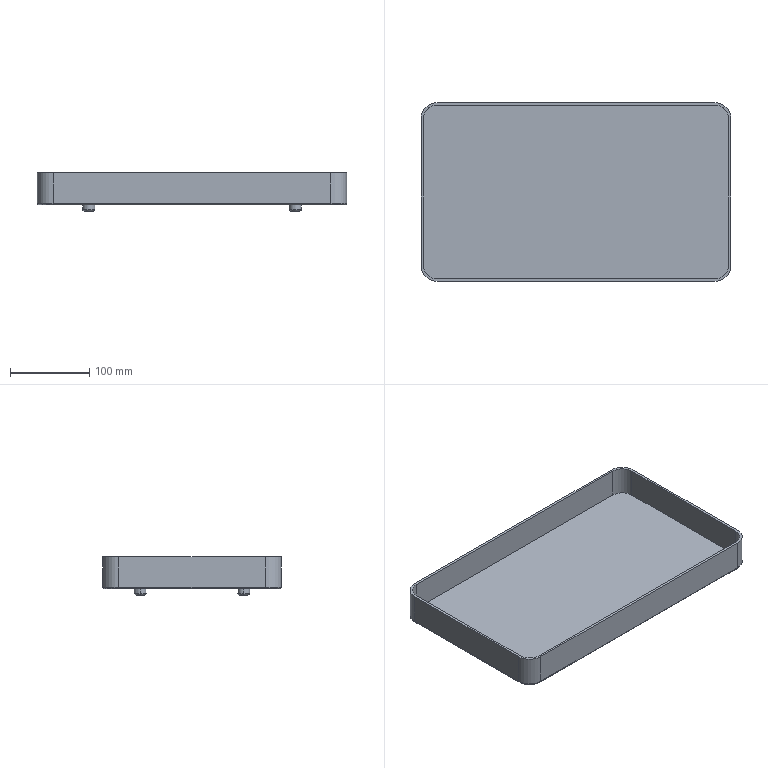Part | SolidWorks | features Fillet 3, Extrusion 1, ICE 1, LPattern 1, Shell 1 | 1 solid | 47 faces | box 390 x 225 x 48 mm | volume 398371 mm3 | cylinder 20 | plane 15 | torus 12 | commonest cylinder face diameters 15 x8 4 x4 34 x4 40 x4
STEP:
#1=CARTESIAN_POINT('',(-122.5,65.,-6.));
#2=VERTEX_POINT('',#1);
#3=CARTESIAN_POINT('',(-137.5,65.,-6.));
#4=VERTEX_POINT('',#3);
#5=CARTESIAN_POINT('',(-130.,65.,-6.));
#6=DIRECTION('',(0.,0.,1.));
#7=DIRECTION('',(-1.,0.,0.));
#8=AXIS2_PLACEMENT_3D('',#5,#6,#7);
#9=CIRCLE('',#8,7.5);
#10=EDGE_CURVE('',#2,#4,#9,.T.);
#11=ORIENTED_EDGE('',*,*,#10,.F.);
#12=CARTESIAN_POINT('',(-124.5,65.,-8.));
#13=VERTEX_POINT('',#12);
#14=CARTESIAN_POINT('',(-124.5,65.,-6.));
#15=DIRECTION('',(0.,1.,0.));
#16=DIRECTION('',(-1.,0.,0.));
#17=AXIS2_PLACEMENT_3D('',#14,#15,#16);
#18=CIRCLE('',#17,2.);
#19=EDGE_CURVE('',#2,#13,#18,.T.);
#20=ORIENTED_EDGE('',*,*,#19,.T.);
#21=CARTESIAN_POINT('',(-135.5,65.,-8.));
#22=VERTEX_POINT('',#21);
#23=CARTESIAN_POINT('',(-130.,65.,-8.));
#24=DIRECTION('',(0.,0.,-1.));
#25=DIRECTION('',(-1.,0.,0.));
#26=AXIS2_PLACEMENT_3D('',#23,#24,#25);
#27=CIRCLE('',#26,5.5);
#28=EDGE_CURVE('',#22,#13,#27,.T.);
#29=ORIENTED_EDGE('',*,*,#28,.F.);
#30=CARTESIAN_POINT('',(-135.5,65.,-6.));
#31=DIRECTION('',(0.,-1.,0.));
#32=DIRECTION('',(0.,0.,-1.));
#33=AXIS2_PLACEMENT_3D('',#30,#31,#32);
#34=CIRCLE('',#33,2.);
#35=EDGE_CURVE('',#4,#22,#34,.T.);
#36=ORIENTED_EDGE('',*,*,#35,.F.);
#37=EDGE_LOOP('',(#11,#20,#29,#36));
#38=FACE_OUTER_BOUND('',#37,.T.);
#39=CARTESIAN_POINT('',(-130.,65.,-6.));
#40=DIRECTION('',(0.,0.,-1.));
#41=DIRECTION('',(-1.,0.,0.));
#42=AXIS2_PLACEMENT_3D('',#39,#40,#41);
#43=TOROIDAL_SURFACE('',#42,5.5,2.);
#44=ADVANCED_FACE('',(#38),#43,.T.);
#45=ORIENTED_EDGE('',*,*,#10,.T.);
#46=CARTESIAN_POINT('',(-137.5,65.,0.));
#47=VERTEX_POINT('',#46);
#48=CARTESIAN_POINT('',(-137.5,65.,-8.));
#49=DIRECTION('',(0.,0.,1.));
#50=VECTOR('',#49,1000.);
#51=LINE('',#48,#50);
#52=EDGE_CURVE('',#4,#47,#51,.T.);
#53=ORIENTED_EDGE('',*,*,#52,.T.);
#54=CARTESIAN_POINT('',(-122.5,65.,0.));
#55=VERTEX_POINT('',#54);
#56=CARTESIAN_POINT('',(-130.,65.,0.));
#57=DIRECTION('',(0.,0.,-1.));
#58=DIRECTION('',(-1.,0.,0.));
#59=AXIS2_PLACEMENT_3D('',#56,#57,#58);
#60=CIRCLE('',#59,7.5);
#61=EDGE_CURVE('',#47,#55,#60,.T.);
#62=ORIENTED_EDGE('',*,*,#61,.T.);
#63=CARTESIAN_POINT('',(-122.5,65.,-8.));
#64=DIRECTION('',(0.,0.,1.));
#65=VECTOR('',#64,1000.);
#66=LINE('',#63,#65);
#67=EDGE_CURVE('',#2,#55,#66,.T.);
#68=ORIENTED_EDGE('',*,*,#67,.F.);
#69=EDGE_LOOP('',(#45,#53,#62,#68));
#70=FACE_OUTER_BOUND('',#69,.T.);
#71=CARTESIAN_POINT('',(-130.,65.,-8.));
#72=DIRECTION('',(0.,0.,1.));
#73=DIRECTION('',(1.,0.,0.));
#74=AXIS2_PLACEMENT_3D('',#71,#72,#73);
#75=CYLINDRICAL_SURFACE('',#74,7.5);
#76=ADVANCED_FACE('',(#70),#75,.T.);
#77=CARTESIAN_POINT('',(137.5,65.,-6.));
#78=VERTEX_POINT('',#77);
#79=CARTESIAN_POINT('',(122.5,65.,-6.));
#80=VERTEX_POINT('',#79);
#81=CARTESIAN_POINT('',(130.,65.,-6.));
#82=DIRECTION('',(0.,0.,1.));
#83=DIRECTION('',(-1.,0.,0.));
#84=AXIS2_PLACEMENT_3D('',#81,#82,#83);
#85=CIRCLE('',#84,7.5);
#86=EDGE_CURVE('',#78,#80,#85,.T.);
#87=ORIENTED_EDGE('',*,*,#86,.F.);
#88=CARTESIAN_POINT('',(135.5,65.,-8.));
#89=VERTEX_POINT('',#88);
#90=CARTESIAN_POINT('',(135.5,65.,-6.));
#91=DIRECTION('',(0.,1.,0.));
#92=DIRECTION('',(-1.,0.,0.));
#93=AXIS2_PLACEMENT_3D('',#90,#91,#92);
#94=CIRCLE('',#93,2.);
#95=EDGE_CURVE('',#78,#89,#94,.T.);
#96=ORIENTED_EDGE('',*,*,#95,.T.);
#97=CARTESIAN_POINT('',(124.5,65.,-8.));
#98=VERTEX_POINT('',#97);
#99=CARTESIAN_POINT('',(130.,65.,-8.));
#100=DIRECTION('',(0.,0.,-1.));
#101=DIRECTION('',(-1.,0.,0.));
#102=AXIS2_PLACEMENT_3D('',#99,#100,#101);
#103=CIRCLE('',#102,5.5);
#104=EDGE_CURVE('',#98,#89,#103,.T.);
#105=ORIENTED_EDGE('',*,*,#104,.F.);
#106=CARTESIAN_POINT('',(124.5,65.,-6.));
#107=DIRECTION('',(0.,-1.,0.));
#108=DIRECTION('',(0.,0.,-1.));
#109=AXIS2_PLACEMENT_3D('',#106,#107,#108);
#110=CIRCLE('',#109,2.);
#111=EDGE_CURVE('',#80,#98,#110,.T.);
#112=ORIENTED_EDGE('',*,*,#111,.F.);
#113=EDGE_LOOP('',(#87,#96,#105,#112));
#114=FACE_OUTER_BOUND('',#113,.T.);
#115=CARTESIAN_POINT('',(130.,65.,-6.));
#116=DIRECTION('',(0.,0.,-1.));
#117=DIRECTION('',(-1.,0.,0.));
#118=AXIS2_PLACEMENT_3D('',#115,#116,#117);
#119=TOROIDAL_SURFACE('',#118,5.5,2.);
#120=ADVANCED_FACE('',(#114),#119,.T.);
#121=ORIENTED_EDGE('',*,*,#86,.T.);
#122=CARTESIAN_POINT('',(122.5,65.,0.));
#123=VERTEX_POINT('',#122);
#124=CARTESIAN_POINT('',(122.5,65.,-8.));
#125=DIRECTION('',(0.,0.,1.));
#126=VECTOR('',#125,1000.);
#127=LINE('',#124,#126);
#128=EDGE_CURVE('',#80,#123,#127,.T.);
#129=ORIENTED_EDGE('',*,*,#128,.T.);
#130=CARTESIAN_POINT('',(137.5,65.,0.));
#131=VERTEX_POINT('',#130);
#132=CARTESIAN_POINT('',(130.,65.,0.));
#133=DIRECTION('',(0.,0.,-1.));
#134=DIRECTION('',(-1.,0.,0.));
#135=AXIS2_PLACEMENT_3D('',#132,#133,#134);
#136=CIRCLE('',#135,7.5);
#137=EDGE_CURVE('',#123,#131,#136,.T.);
#138=ORIENTED_EDGE('',*,*,#137,.T.);
#139=CARTESIAN_POINT('',(137.5,65.,-8.));
#140=DIRECTION('',(0.,0.,1.));
#141=VECTOR('',#140,1000.);
#142=LINE('',#139,#141);
#143=EDGE_CURVE('',#78,#131,#142,.T.);
#144=ORIENTED_EDGE('',*,*,#143,.F.);
#145=EDGE_LOOP('',(#121,#129,#138,#144));
#146=FACE_OUTER_BOUND('',#145,.T.);
#147=CARTESIAN_POINT('',(130.,65.,-8.));
#148=DIRECTION('',(0.,0.,1.));
#149=DIRECTION('',(1.,0.,0.));
#150=AXIS2_PLACEMENT_3D('',#147,#148,#149);
#151=CYLINDRICAL_SURFACE('',#150,7.5);
#152=ADVANCED_FACE('',(#146),#151,.T.);
#153=CARTESIAN_POINT('',(137.5,-65.,-6.));
#154=VERTEX_POINT('',#153);
#155=CARTESIAN_POINT('',(122.5,-65.,-6.));
#156=VERTEX_POINT('',#155);
#157=CARTESIAN_POINT('',(130.,-65.,-6.));
#158=DIRECTION('',(0.,0.,1.));
#159=DIRECTION('',(-1.,0.,0.));
#160=AXIS2_PLACEMENT_3D('',#157,#158,#159);
#161=CIRCLE('',#160,7.5);
#162=EDGE_CURVE('',#154,#156,#161,.T.);
#163=ORIENTED_EDGE('',*,*,#162,.T.);
#164=CARTESIAN_POINT('',(122.5,-65.,0.));
#165=VERTEX_POINT('',#164);
#166=CARTESIAN_POINT('',(122.5,-65.,-8.));
#167=DIRECTION('',(0.,0.,1.));
#168=VECTOR('',#167,1000.);
#169=LINE('',#166,#168);
#170=EDGE_CURVE('',#156,#165,#169,.T.);
#171=ORIENTED_EDGE('',*,*,#170,.T.);
#172=CARTESIAN_POINT('',(137.5,-65.,0.));
#173=VERTEX_POINT('',#172);
#174=CARTESIAN_POINT('',(130.,-65.,0.));
#175=DIRECTION('',(0.,0.,-1.));
#176=DIRECTION('',(-1.,0.,0.));
#177=AXIS2_PLACEMENT_3D('',#174,#175,#176);
#178=CIRCLE('',#177,7.5);
#179=EDGE_CURVE('',#165,#173,#178,.T.);
#180=ORIENTED_EDGE('',*,*,#179,.T.);
#181=CARTESIAN_POINT('',(137.5,-65.,-8.));
#182=DIRECTION('',(0.,0.,1.));
#183=VECTOR('',#182,1000.);
#184=LINE('',#181,#183);
#185=EDGE_CURVE('',#154,#173,#184,.T.);
#186=ORIENTED_EDGE('',*,*,#185,.F.);
#187=EDGE_LOOP('',(#163,#171,#180,#186));
#188=FACE_OUTER_BOUND('',#187,.T.);
#189=CARTESIAN_POINT('',(130.,-65.,-8.));
#190=DIRECTION('',(0.,0.,1.));
#191=DIRECTION('',(1.,0.,0.));
#192=AXIS2_PLACEMENT_3D('',#189,#190,#191);
#193=CYLINDRICAL_SURFACE('',#192,7.5);
#194=ADVANCED_FACE('',(#188),#193,.T.);
#195=ORIENTED_EDGE('',*,*,#162,.F.);
#196=CARTESIAN_POINT('',(135.5,-65.,-8.));
#197=VERTEX_POINT('',#196);
#198=CARTESIAN_POINT('',(135.5,-65.,-6.));
#199=DIRECTION('',(0.,1.,0.));
#200=DIRECTION('',(-1.,0.,0.));
#201=AXIS2_PLACEMENT_3D('',#198,#199,#200);
#202=CIRCLE('',#201,2.);
#203=EDGE_CURVE('',#154,#197,#202,.T.);
#204=ORIENTED_EDGE('',*,*,#203,.T.);
#205=CARTESIAN_POINT('',(124.5,-65.,-8.));
#206=VERTEX_POINT('',#205);
#207=CARTESIAN_POINT('',(130.,-65.,-8.));
#208=DIRECTION('',(0.,0.,-1.));
#209=DIRECTION('',(-1.,0.,0.));
#210=AXIS2_PLACEMENT_3D('',#207,#208,#209);
#211=CIRCLE('',#210,5.5);
#212=EDGE_CURVE('',#206,#197,#211,.T.);
#213=ORIENTED_EDGE('',*,*,#212,.F.);
#214=CARTESIAN_POINT('',(124.5,-65.,-6.));
#215=DIRECTION('',(0.,-1.,0.));
#216=DIRECTION('',(0.,0.,-1.));
#217=AXIS2_PLACEMENT_3D('',#214,#215,#216);
#218=CIRCLE('',#217,2.);
#219=EDGE_CURVE('',#156,#206,#218,.T.);
#220=ORIENTED_EDGE('',*,*,#219,.F.);
#221=EDGE_LOOP('',(#195,#204,#213,#220));
#222=FACE_OUTER_BOUND('',#221,.T.);
#223=CARTESIAN_POINT('',(130.,-65.,-6.));
#224=DIRECTION('',(0.,0.,-1.));
#225=DIRECTION('',(-1.,0.,0.));
#226=AXIS2_PLACEMENT_3D('',#223,#224,#225);
#227=TOROIDAL_SURFACE('',#226,5.5,2.);
#228=ADVANCED_FACE('',(#222),#227,.T.);
#229=CARTESIAN_POINT('',(-122.5,-65.,-6.));
#230=VERTEX_POINT('',#229);
#231=CARTESIAN_POINT('',(-137.5,-65.,-6.));
#232=VERTEX_POINT('',#231);
#233=CARTESIAN_POINT('',(-130.,-65.,-6.));
#234=DIRECTION('',(0.,0.,1.));
#235=DIRECTION('',(-1.,0.,0.));
#236=AXIS2_PLACEMENT_3D('',#233,#234,#235);
#237=CIRCLE('',#236,7.5);
#238=EDGE_CURVE('',#230,#232,#237,.T.);
#239=ORIENTED_EDGE('',*,*,#238,.T.);
#240=CARTESIAN_POINT('',(-137.5,-65.,0.));
#241=VERTEX_POINT('',#240);
#242=CARTESIAN_POINT('',(-137.5,-65.,-8.));
#243=DIRECTION('',(0.,0.,1.));
#244=VECTOR('',#243,1000.);
#245=LINE('',#242,#244);
#246=EDGE_CURVE('',#232,#241,#245,.T.);
#247=ORIENTED_EDGE('',*,*,#246,.T.);
#248=CARTESIAN_POINT('',(-122.5,-65.,0.));
#249=VERTEX_POINT('',#248);
#250=CARTESIAN_POINT('',(-130.,-65.,0.));
#251=DIRECTION('',(0.,0.,-1.));
#252=DIRECTION('',(-1.,0.,0.));
#253=AXIS2_PLACEMENT_3D('',#250,#251,#252);
#254=CIRCLE('',#253,7.5);
#255=EDGE_CURVE('',#241,#249,#254,.T.);
#256=ORIENTED_EDGE('',*,*,#255,.T.);
#257=CARTESIAN_POINT('',(-122.5,-65.,-8.));
#258=DIRECTION('',(0.,0.,1.));
#259=VECTOR('',#258,1000.);
#260=LINE('',#257,#259);
#261=EDGE_CURVE('',#230,#249,#260,.T.);
#262=ORIENTED_EDGE('',*,*,#261,.F.);
#263=EDGE_LOOP('',(#239,#247,#256,#262));
#264=FACE_OUTER_BOUND('',#263,.T.);
#265=CARTESIAN_POINT('',(-130.,-65.,-8.));
#266=DIRECTION('',(0.,0.,1.));
#267=DIRECTION('',(1.,0.,0.));
#268=AXIS2_PLACEMENT_3D('',#265,#266,#267);
#269=CYLINDRICAL_SURFACE('',#268,7.5);
#270=ADVANCED_FACE('',(#264),#269,.T.);
#271=ORIENTED_EDGE('',*,*,#238,.F.);
#272=CARTESIAN_POINT('',(-124.5,-65.,-8.));
#273=VERTEX_POINT('',#272);
#274=CARTESIAN_POINT('',(-124.5,-65.,-6.));
#275=DIRECTION('',(0.,1.,0.));
#276=DIRECTION('',(-1.,0.,0.));
#277=AXIS2_PLACEMENT_3D('',#274,#275,#276);
#278=CIRCLE('',#277,2.);
#279=EDGE_CURVE('',#230,#273,#278,.T.);
#280=ORIENTED_EDGE('',*,*,#279,.T.);
#281=CARTESIAN_POINT('',(-135.5,-65.,-8.));
#282=VERTEX_POINT('',#281);
#283=CARTESIAN_POINT('',(-130.,-65.,-8.));
#284=DIRECTION('',(0.,0.,-1.));
#285=DIRECTION('',(-1.,0.,0.));
#286=AXIS2_PLACEMENT_3D('',#283,#284,#285);
#287=CIRCLE('',#286,5.5);
#288=EDGE_CURVE('',#282,#273,#287,.T.);
#289=ORIENTED_EDGE('',*,*,#288,.F.);
#290=CARTESIAN_POINT('',(-135.5,-65.,-6.));
#291=DIRECTION('',(0.,-1.,0.));
#292=DIRECTION('',(0.,0.,-1.));
#293=AXIS2_PLACEMENT_3D('',#290,#291,#292);
#294=CIRCLE('',#293,2.);
#295=EDGE_CURVE('',#232,#282,#294,.T.);
#296=ORIENTED_EDGE('',*,*,#295,.F.);
#297=EDGE_LOOP('',(#271,#280,#289,#296));
#298=FACE_OUTER_BOUND('',#297,.T.);
#299=CARTESIAN_POINT('',(-130.,-65.,-6.));
#300=DIRECTION('',(0.,0.,-1.));
#301=DIRECTION('',(-1.,0.,0.));
#302=AXIS2_PLACEMENT_3D('',#299,#300,#301);
#303=TOROIDAL_SURFACE('',#302,5.5,2.);
#304=ADVANCED_FACE('',(#298),#303,.T.);
#305=ORIENTED_EDGE('',*,*,#279,.F.);
#306=CARTESIAN_POINT('',(-130.,-65.,-6.));
#307=DIRECTION('',(0.,0.,1.));
#308=DIRECTION('',(-1.,0.,0.));
#309=AXIS2_PLACEMENT_3D('',#306,#307,#308);
#310=CIRCLE('',#309,7.5);
#311=EDGE_CURVE('',#232,#230,#310,.T.);
#312=ORIENTED_EDGE('',*,*,#311,.F.);
#313=ORIENTED_EDGE('',*,*,#295,.T.);
#314=CARTESIAN_POINT('',(-130.,-65.,-8.));
#315=DIRECTION('',(0.,0.,-1.));
#316=DIRECTION('',(-1.,0.,0.));
#317=AXIS2_PLACEMENT_3D('',#314,#315,#316);
#318=CIRCLE('',#317,5.5);
#319=EDGE_CURVE('',#273,#282,#318,.T.);
#320=ORIENTED_EDGE('',*,*,#319,.F.);
#321=EDGE_LOOP('',(#305,#312,#313,#320));
#322=FACE_OUTER_BOUND('',#321,.T.);
#323=CARTESIAN_POINT('',(-130.,-65.,-6.));
#324=DIRECTION('',(0.,0.,-1.));
#325=DIRECTION('',(-1.,0.,0.));
#326=AXIS2_PLACEMENT_3D('',#323,#324,#325);
#327=TOROIDAL_SURFACE('',#326,5.5,2.);
#328=ADVANCED_FACE('',(#322),#327,.T.);
#329=ORIENTED_EDGE('',*,*,#288,.T.);
#330=ORIENTED_EDGE('',*,*,#319,.T.);
#331=EDGE_LOOP('',(#329,#330));
#332=FACE_OUTER_BOUND('',#331,.T.);
#333=CARTESIAN_POINT('',(-130.,-65.,-8.));
#334=DIRECTION('',(0.,0.,-1.));
#335=DIRECTION('',(-1.,0.,0.));
#336=AXIS2_PLACEMENT_3D('',#333,#334,#335);
#337=PLANE('',#336);
#338=ADVANCED_FACE('',(#332),#337,.T.);
#339=ORIENTED_EDGE('',*,*,#246,.F.);
#340=ORIENTED_EDGE('',*,*,#311,.T.);
#341=ORIENTED_EDGE('',*,*,#261,.T.);
#342=CARTESIAN_POINT('',(-130.,-65.,0.));
#343=DIRECTION('',(0.,0.,-1.));
#344=DIRECTION('',(-1.,0.,0.));
#345=AXIS2_PLACEMENT_3D('',#342,#343,#344);
#346=CIRCLE('',#345,7.5);
#347=EDGE_CURVE('',#249,#241,#346,.T.);
#348=ORIENTED_EDGE('',*,*,#347,.T.);
#349=EDGE_LOOP('',(#339,#340,#341,#348));
#350=FACE_OUTER_BOUND('',#349,.T.);
#351=CARTESIAN_POINT('',(-130.,-65.,-8.));
#352=DIRECTION('',(0.,0.,1.));
#353=DIRECTION('',(1.,0.,0.));
#354=AXIS2_PLACEMENT_3D('',#351,#352,#353);
#355=CYLINDRICAL_SURFACE('',#354,7.5);
#356=ADVANCED_FACE('',(#350),#355,.T.);
#357=ORIENTED_EDGE('',*,*,#203,.F.);
#358=CARTESIAN_POINT('',(130.,-65.,-6.));
#359=DIRECTION('',(0.,0.,1.));
#360=DIRECTION('',(-1.,0.,0.));
#361=AXIS2_PLACEMENT_3D('',#358,#359,#360);
#362=CIRCLE('',#361,7.5);
#363=EDGE_CURVE('',#156,#154,#362,.T.);
#364=ORIENTED_EDGE('',*,*,#363,.F.);
#365=ORIENTED_EDGE('',*,*,#219,.T.);
#366=CARTESIAN_POINT('',(130.,-65.,-8.));
#367=DIRECTION('',(0.,0.,-1.));
#368=DIRECTION('',(-1.,0.,0.));
#369=AXIS2_PLACEMENT_3D('',#366,#367,#368);
#370=CIRCLE('',#369,5.5);
#371=EDGE_CURVE('',#197,#206,#370,.T.);
#372=ORIENTED_EDGE('',*,*,#371,.F.);
#373=EDGE_LOOP('',(#357,#364,#365,#372));
#374=FACE_OUTER_BOUND('',#373,.T.);
#375=CARTESIAN_POINT('',(130.,-65.,-6.));
#376=DIRECTION('',(0.,0.,-1.));
#377=DIRECTION('',(-1.,0.,0.));
#378=AXIS2_PLACEMENT_3D('',#375,#376,#377);
#379=TOROIDAL_SURFACE('',#378,5.5,2.);
#380=ADVANCED_FACE('',(#374),#379,.T.);
#381=ORIENTED_EDGE('',*,*,#212,.T.);
#382=ORIENTED_EDGE('',*,*,#371,.T.);
#383=EDGE_LOOP('',(#381,#382));
#384=FACE_OUTER_BOUND('',#383,.T.);
#385=CARTESIAN_POINT('',(130.,-65.,-8.));
#386=DIRECTION('',(0.,0.,-1.));
#387=DIRECTION('',(-1.,0.,0.));
#388=AXIS2_PLACEMENT_3D('',#385,#386,#387);
#389=PLANE('',#388);
#390=ADVANCED_FACE('',(#384),#389,.T.);
#391=ORIENTED_EDGE('',*,*,#170,.F.);
#392=ORIENTED_EDGE('',*,*,#363,.T.);
#393=ORIENTED_EDGE('',*,*,#185,.T.);
#394=CARTESIAN_POINT('',(130.,-65.,0.));
#395=DIRECTION('',(0.,0.,-1.));
#396=DIRECTION('',(-1.,0.,0.));
#397=AXIS2_PLACEMENT_3D('',#394,#395,#396);
#398=CIRCLE('',#397,7.5);
#399=EDGE_CURVE('',#173,#165,#398,.T.);
#400=ORIENTED_EDGE('',*,*,#399,.T.);
#401=EDGE_LOOP('',(#391,#392,#393,#400));
#402=FACE_OUTER_BOUND('',#401,.T.);
#403=CARTESIAN_POINT('',(130.,-65.,-8.));
#404=DIRECTION('',(0.,0.,1.));
#405=DIRECTION('',(1.,0.,0.));
#406=AXIS2_PLACEMENT_3D('',#403,#404,#405);
#407=CYLINDRICAL_SURFACE('',#406,7.5);
#408=ADVANCED_FACE('',(#402),#407,.T.);
#409=CARTESIAN_POINT('',(195.,-92.5,40.));
#410=VERTEX_POINT('',#409);
#411=CARTESIAN_POINT('',(195.,-92.5,2.));
#412=VERTEX_POINT('',#411);
#413=CARTESIAN_POINT('',(195.,-92.5,40.));
#414=DIRECTION('',(0.,0.,-1.));
#415=VECTOR('',#414,1000.);
#416=LINE('',#413,#415);
#417=EDGE_CURVE('',#410,#412,#416,.T.);
#418=ORIENTED_EDGE('',*,*,#417,.T.);
#419=CARTESIAN_POINT('',(195.,92.5,2.));
#420=VERTEX_POINT('',#419);
#421=CARTESIAN_POINT('',(195.,92.5,2.));
#422=DIRECTION('',(0.,1.,0.));
#423=VECTOR('',#422,1000.);
#424=LINE('',#421,#423);
#425=EDGE_CURVE('',#412,#420,#424,.T.);
#426=ORIENTED_EDGE('',*,*,#425,.T.);
#427=CARTESIAN_POINT('',(195.,92.5,40.));
#428=VERTEX_POINT('',#427);
#429=CARTESIAN_POINT('',(195.,92.5,40.));
#430=DIRECTION('',(0.,0.,1.));
#431=VECTOR('',#430,1000.);
#432=LINE('',#429,#431);
#433=EDGE_CURVE('',#420,#428,#432,.T.);
#434=ORIENTED_EDGE('',*,*,#433,.T.);
#435=CARTESIAN_POINT('',(195.,-112.5,40.));
#436=DIRECTION('',(0.,1.,0.));
#437=VECTOR('',#436,1000.);
#438=LINE('',#435,#437);
#439=EDGE_CURVE('',#410,#428,#438,.T.);
#440=ORIENTED_EDGE('',*,*,#439,.F.);
#441=EDGE_LOOP('',(#418,#426,#434,#440));
#442=FACE_OUTER_BOUND('',#441,.T.);
#443=CARTESIAN_POINT('',(195.,-112.5,40.));
#444=DIRECTION('',(-1.,0.,0.));
#445=DIRECTION('',(0.,0.,1.));
#446=AXIS2_PLACEMENT_3D('',#443,#444,#445);
#447=PLANE('',#446);
#448=ADVANCED_FACE('',(#442),#447,.F.);
#449=CARTESIAN_POINT('',(175.,112.5,40.));
#450=VERTEX_POINT('',#449);
#451=CARTESIAN_POINT('',(175.,112.5,2.));
#452=VERTEX_POINT('',#451);
#453=CARTESIAN_POINT('',(175.,112.5,40.));
#454=DIRECTION('',(0.,0.,-1.));
#455=VECTOR('',#454,1000.);
#456=LINE('',#453,#455);
#457=EDGE_CURVE('',#450,#452,#456,.T.);
#458=ORIENTED_EDGE('',*,*,#457,.T.);
#459=CARTESIAN_POINT('',(-175.,112.5,2.));
#460=VERTEX_POINT('',#459);
#461=CARTESIAN_POINT('',(-175.,112.5,2.));
#462=DIRECTION('',(-1.,0.,0.));
#463=VECTOR('',#462,1000.);
#464=LINE('',#461,#463);
#465=EDGE_CURVE('',#452,#460,#464,.T.);
#466=ORIENTED_EDGE('',*,*,#465,.T.);
#467=CARTESIAN_POINT('',(-175.,112.5,40.));
#468=VERTEX_POINT('',#467);
#469=CARTESIAN_POINT('',(-175.,112.5,40.));
#470=DIRECTION('',(0.,0.,1.));
#471=VECTOR('',#470,1000.);
#472=LINE('',#469,#471);
#473=EDGE_CURVE('',#460,#468,#472,.T.);
#474=ORIENTED_EDGE('',*,*,#473,.T.);
#475=CARTESIAN_POINT('',(-195.,112.5,40.));
#476=DIRECTION('',(-1.,0.,0.));
#477=VECTOR('',#476,1000.);
#478=LINE('',#475,#477);
#479=EDGE_CURVE('',#450,#468,#478,.T.);
#480=ORIENTED_EDGE('',*,*,#479,.F.);
#481=EDGE_LOOP('',(#458,#466,#474,#480));
#482=FACE_OUTER_BOUND('',#481,.T.);
#483=CARTESIAN_POINT('',(-195.,112.5,40.));
#484=DIRECTION('',(0.,-1.,0.));
#485=DIRECTION('',(0.,0.,-1.));
#486=AXIS2_PLACEMENT_3D('',#483,#484,#485);
#487=PLANE('',#486);
#488=ADVANCED_FACE('',(#482),#487,.F.);
#489=CARTESIAN_POINT('',(-195.,92.5,40.));
#490=VERTEX_POINT('',#489);
#491=CARTESIAN_POINT('',(-195.,92.5,2.));
#492=VERTEX_POINT('',#491);
#493=CARTESIAN_POINT('',(-195.,92.5,40.));
#494=DIRECTION('',(0.,0.,-1.));
#495=VECTOR('',#494,1000.);
#496=LINE('',#493,#495);
#497=EDGE_CURVE('',#490,#492,#496,.T.);
#498=ORIENTED_EDGE('',*,*,#497,.T.);
#499=CARTESIAN_POINT('',(-195.,-92.5,2.));
#500=VERTEX_POINT('',#499);
#501=CARTESIAN_POINT('',(-195.,-92.5,2.));
#502=DIRECTION('',(0.,-1.,0.));
#503=VECTOR('',#502,1000.);
#504=LINE('',#501,#503);
#505=EDGE_CURVE('',#492,#500,#504,.T.);
#506=ORIENTED_EDGE('',*,*,#505,.T.);
#507=CARTESIAN_POINT('',(-195.,-92.5,40.));
#508=VERTEX_POINT('',#507);
#509=CARTESIAN_POINT('',(-195.,-92.5,40.));
#510=DIRECTION('',(0.,0.,1.));
#511=VECTOR('',#510,1000.);
#512=LINE('',#509,#511);
#513=EDGE_CURVE('',#500,#508,#512,.T.);
#514=ORIENTED_EDGE('',*,*,#513,.T.);
#515=CARTESIAN_POINT('',(-195.,-112.5,40.));
#516=DIRECTION('',(0.,-1.,0.));
#517=VECTOR('',#516,1000.);
#518=LINE('',#515,#517);
#519=EDGE_CURVE('',#490,#508,#518,.T.);
#520=ORIENTED_EDGE('',*,*,#519,.F.);
#521=EDGE_LOOP('',(#498,#506,#514,#520));
#522=FACE_OUTER_BOUND('',#521,.T.);
#523=CARTESIAN_POINT('',(-195.,-112.5,40.));
#524=DIRECTION('',(1.,0.,0.));
#525=DIRECTION('',(0.,0.,-1.));
#526=AXIS2_PLACEMENT_3D('',#523,#524,#525);
#527=PLANE('',#526);
#528=ADVANCED_FACE('',(#522),#527,.F.);
#529=CARTESIAN_POINT('',(-175.,-112.5,40.));
#530=VERTEX_POINT('',#529);
#531=CARTESIAN_POINT('',(-175.,-112.5,2.));
#532=VERTEX_POINT('',#531);
#533=CARTESIAN_POINT('',(-175.,-112.5,40.));
#534=DIRECTION('',(0.,0.,-1.));
#535=VECTOR('',#534,1000.);
#536=LINE('',#533,#535);
#537=EDGE_CURVE('',#530,#532,#536,.T.);
#538=ORIENTED_EDGE('',*,*,#537,.T.);
#539=CARTESIAN_POINT('',(175.,-112.5,2.));
#540=VERTEX_POINT('',#539);
#541=CARTESIAN_POINT('',(175.,-112.5,2.));
#542=DIRECTION('',(1.,0.,0.));
#543=VECTOR('',#542,1000.);
#544=LINE('',#541,#543);
#545=EDGE_CURVE('',#532,#540,#544,.T.);
#546=ORIENTED_EDGE('',*,*,#545,.T.);
#547=CARTESIAN_POINT('',(175.,-112.5,40.));
#548=VERTEX_POINT('',#547);
#549=CARTESIAN_POINT('',(175.,-112.5,40.));
#550=DIRECTION('',(0.,0.,1.));
#551=VECTOR('',#550,1000.);
#552=LINE('',#549,#551);
#553=EDGE_CURVE('',#540,#548,#552,.T.);
#554=ORIENTED_EDGE('',*,*,#553,.T.);
#555=CARTESIAN_POINT('',(-195.,-112.5,40.));
#556=DIRECTION('',(1.,0.,0.));
#557=VECTOR('',#556,1000.);
#558=LINE('',#555,#557);
#559=EDGE_CURVE('',#530,#548,#558,.T.);
#560=ORIENTED_EDGE('',*,*,#559,.F.);
#561=EDGE_LOOP('',(#538,#546,#554,#560));
#562=FACE_OUTER_BOUND('',#561,.T.);
#563=CARTESIAN_POINT('',(-195.,-112.5,40.));
#564=DIRECTION('',(0.,1.,0.));
#565=DIRECTION('',(0.,0.,1.));
#566=AXIS2_PLACEMENT_3D('',#563,#564,#565);
#567=PLANE('',#566);
#568=ADVANCED_FACE('',(#562),#567,.F.);
#569=CARTESIAN_POINT('',(-175.,-109.5,40.));
#570=VERTEX_POINT('',#569);
#571=CARTESIAN_POINT('',(175.,-109.5,40.));
#572=VERTEX_POINT('',#571);
#573=CARTESIAN_POINT('',(0.,-109.5,40.));
#574=DIRECTION('',(1.,0.,0.));
#575=VECTOR('',#574,1000.);
#576=LINE('',#573,#575);
#577=EDGE_CURVE('',#570,#572,#576,.T.);
#578=ORIENTED_EDGE('',*,*,#577,.F.);
#579=CARTESIAN_POINT('',(-192.,-92.5,40.));
#580=VERTEX_POINT('',#579);
#581=CARTESIAN_POINT('',(-175.,-92.5,40.));
#582=DIRECTION('',(0.,0.,1.));
#583=DIRECTION('',(-1.,0.,0.));
#584=AXIS2_PLACEMENT_3D('',#581,#582,#583);
#585=CIRCLE('',#584,17.);
#586=EDGE_CURVE('',#580,#570,#585,.T.);
#587=ORIENTED_EDGE('',*,*,#586,.F.);
#588=CARTESIAN_POINT('',(-192.,92.5,40.));
#589=VERTEX_POINT('',#588);
#590=CARTESIAN_POINT('',(-192.,0.,40.));
#591=DIRECTION('',(0.,-1.,0.));
#592=VECTOR('',#591,1000.);
#593=LINE('',#590,#592);
#594=EDGE_CURVE('',#589,#580,#593,.T.);
#595=ORIENTED_EDGE('',*,*,#594,.F.);
#596=CARTESIAN_POINT('',(-175.,109.5,40.));
#597=VERTEX_POINT('',#596);
#598=CARTESIAN_POINT('',(-175.,92.5,40.));
#599=DIRECTION('',(0.,0.,1.));
#600=DIRECTION('',(-1.,0.,0.));
#601=AXIS2_PLACEMENT_3D('',#598,#599,#600);
#602=CIRCLE('',#601,17.);
#603=EDGE_CURVE('',#597,#589,#602,.T.);
#604=ORIENTED_EDGE('',*,*,#603,.F.);
#605=CARTESIAN_POINT('',(175.,109.5,40.));
#606=VERTEX_POINT('',#605);
#607=CARTESIAN_POINT('',(0.,109.5,40.));
#608=DIRECTION('',(-1.,0.,0.));
#609=VECTOR('',#608,1000.);
#610=LINE('',#607,#609);
#611=EDGE_CURVE('',#606,#597,#610,.T.);
#612=ORIENTED_EDGE('',*,*,#611,.F.);
#613=CARTESIAN_POINT('',(192.,92.5,40.));
#614=VERTEX_POINT('',#613);
#615=CARTESIAN_POINT('',(175.,92.5,40.));
#616=DIRECTION('',(0.,0.,1.));
#617=DIRECTION('',(-1.,0.,0.));
#618=AXIS2_PLACEMENT_3D('',#615,#616,#617);
#619=CIRCLE('',#618,17.);
#620=EDGE_CURVE('',#614,#606,#619,.T.);
#621=ORIENTED_EDGE('',*,*,#620,.F.);
#622=CARTESIAN_POINT('',(192.,-92.5,40.));
#623=VERTEX_POINT('',#622);
#624=CARTESIAN_POINT('',(192.,0.,40.));
#625=DIRECTION('',(0.,1.,0.));
#626=VECTOR('',#625,1000.);
#627=LINE('',#624,#626);
#628=EDGE_CURVE('',#623,#614,#627,.T.);
#629=ORIENTED_EDGE('',*,*,#628,.F.);
#630=CARTESIAN_POINT('',(175.,-92.5,40.));
#631=DIRECTION('',(0.,0.,1.));
#632=DIRECTION('',(-1.,0.,0.));
#633=AXIS2_PLACEMENT_3D('',#630,#631,#632);
#634=CIRCLE('',#633,17.);
#635=EDGE_CURVE('',#572,#623,#634,.T.);
#636=ORIENTED_EDGE('',*,*,#635,.F.);
#637=EDGE_LOOP('',(#578,#587,#595,#604,#612,#621,#629,#636));
#638=FACE_BOUND('',#637,.T.);
#639=ORIENTED_EDGE('',*,*,#559,.T.);
#640=CARTESIAN_POINT('',(175.,-92.5,40.));
#641=DIRECTION('',(0.,0.,1.));
#642=DIRECTION('',(-1.,0.,0.));
#643=AXIS2_PLACEMENT_3D('',#640,#641,#642);
#644=CIRCLE('',#643,20.);
#645=EDGE_CURVE('',#548,#410,#644,.T.);
#646=ORIENTED_EDGE('',*,*,#645,.T.);
#647=ORIENTED_EDGE('',*,*,#439,.T.);
#648=CARTESIAN_POINT('',(175.,92.5,40.));
#649=DIRECTION('',(0.,0.,1.));
#650=DIRECTION('',(-1.,0.,0.));
#651=AXIS2_PLACEMENT_3D('',#648,#649,#650);
#652=CIRCLE('',#651,20.);
#653=EDGE_CURVE('',#428,#450,#652,.T.);
#654=ORIENTED_EDGE('',*,*,#653,.T.);
#655=ORIENTED_EDGE('',*,*,#479,.T.);
#656=CARTESIAN_POINT('',(-175.,92.5,40.));
#657=DIRECTION('',(0.,0.,1.));
#658=DIRECTION('',(-1.,0.,0.));
#659=AXIS2_PLACEMENT_3D('',#656,#657,#658);
#660=CIRCLE('',#659,20.);
#661=EDGE_CURVE('',#468,#490,#660,.T.);
#662=ORIENTED_EDGE('',*,*,#661,.T.);
#663=ORIENTED_EDGE('',*,*,#519,.T.);
#664=CARTESIAN_POINT('',(-175.,-92.5,40.));
#665=DIRECTION('',(0.,0.,1.));
#666=DIRECTION('',(-1.,0.,0.));
#667=AXIS2_PLACEMENT_3D('',#664,#665,#666);
#668=CIRCLE('',#667,20.);
#669=EDGE_CURVE('',#508,#530,#668,.T.);
#670=ORIENTED_EDGE('',*,*,#669,.T.);
#671=EDGE_LOOP('',(#639,#646,#647,#654,#655,#662,#663,#670));
#672=FACE_OUTER_BOUND('',#671,.T.);
#673=CARTESIAN_POINT('',(0.,0.,40.));
#674=DIRECTION('',(0.,0.,-1.));
#675=DIRECTION('',(-1.,0.,0.));
#676=AXIS2_PLACEMENT_3D('',#673,#674,#675);
#677=PLANE('',#676);
#678=ADVANCED_FACE('',(#638,#672),#677,.F.);
#679=CARTESIAN_POINT('',(-130.,65.,0.));
#680=DIRECTION('',(0.,0.,-1.));
#681=DIRECTION('',(-1.,0.,0.));
#682=AXIS2_PLACEMENT_3D('',#679,#680,#681);
#683=CIRCLE('',#682,7.5);
#684=EDGE_CURVE('',#55,#47,#683,.T.);
#685=ORIENTED_EDGE('',*,*,#684,.F.);
#686=ORIENTED_EDGE('',*,*,#61,.F.);
#687=EDGE_LOOP('',(#685,#686));
#688=FACE_BOUND('',#687,.T.);
#689=CARTESIAN_POINT('',(130.,65.,0.));
#690=DIRECTION('',(0.,0.,-1.));
#691=DIRECTION('',(-1.,0.,0.));
#692=AXIS2_PLACEMENT_3D('',#689,#690,#691);
#693=CIRCLE('',#692,7.5);
#694=EDGE_CURVE('',#131,#123,#693,.T.);
#695=ORIENTED_EDGE('',*,*,#694,.F.);
#696=ORIENTED_EDGE('',*,*,#137,.F.);
#697=EDGE_LOOP('',(#695,#696));
#698=FACE_BOUND('',#697,.T.);
#699=CARTESIAN_POINT('',(-175.,110.5,0.));
#700=VERTEX_POINT('',#699);
#701=CARTESIAN_POINT('',(175.,110.5,0.));
#702=VERTEX_POINT('',#701);
#703=CARTESIAN_POINT('',(175.,110.5,0.));
#704=DIRECTION('',(1.,0.,0.));
#705=VECTOR('',#704,1000.);
#706=LINE('',#703,#705);
#707=EDGE_CURVE('',#700,#702,#706,.T.);
#708=ORIENTED_EDGE('',*,*,#707,.T.);
#709=CARTESIAN_POINT('',(193.,92.5,0.));
#710=VERTEX_POINT('',#709);
#711=CARTESIAN_POINT('',(175.,92.5,0.));
#712=DIRECTION('',(0.,0.,-1.));
#713=DIRECTION('',(-1.,0.,0.));
#714=AXIS2_PLACEMENT_3D('',#711,#712,#713);
#715=CIRCLE('',#714,18.);
#716=EDGE_CURVE('',#702,#710,#715,.T.);
#717=ORIENTED_EDGE('',*,*,#716,.T.);
#718=CARTESIAN_POINT('',(193.,-92.5,0.));
#719=VERTEX_POINT('',#718);
#720=CARTESIAN_POINT('',(193.,-92.5,0.));
#721=DIRECTION('',(0.,-1.,0.));
#722=VECTOR('',#721,1000.);
#723=LINE('',#720,#722);
#724=EDGE_CURVE('',#710,#719,#723,.T.);
#725=ORIENTED_EDGE('',*,*,#724,.T.);
#726=CARTESIAN_POINT('',(175.,-110.5,0.));
#727=VERTEX_POINT('',#726);
#728=CARTESIAN_POINT('',(175.,-92.5,0.));
#729=DIRECTION('',(0.,0.,-1.));
#730=DIRECTION('',(-1.,0.,0.));
#731=AXIS2_PLACEMENT_3D('',#728,#729,#730);
#732=CIRCLE('',#731,18.);
#733=EDGE_CURVE('',#719,#727,#732,.T.);
#734=ORIENTED_EDGE('',*,*,#733,.T.);
#735=CARTESIAN_POINT('',(-175.,-110.5,0.));
#736=VERTEX_POINT('',#735);
#737=CARTESIAN_POINT('',(-175.,-110.5,0.));
#738=DIRECTION('',(-1.,0.,0.));
#739=VECTOR('',#738,1000.);
#740=LINE('',#737,#739);
#741=EDGE_CURVE('',#727,#736,#740,.T.);
#742=ORIENTED_EDGE('',*,*,#741,.T.);
#743=CARTESIAN_POINT('',(-193.,-92.5,0.));
#744=VERTEX_POINT('',#743);
#745=CARTESIAN_POINT('',(-175.,-92.5,0.));
#746=DIRECTION('',(0.,0.,-1.));
#747=DIRECTION('',(-1.,0.,0.));
#748=AXIS2_PLACEMENT_3D('',#745,#746,#747);
#749=CIRCLE('',#748,18.);
#750=EDGE_CURVE('',#736,#744,#749,.T.);
#751=ORIENTED_EDGE('',*,*,#750,.T.);
#752=CARTESIAN_POINT('',(-193.,92.5,0.));
#753=VERTEX_POINT('',#752);
#754=CARTESIAN_POINT('',(-193.,92.5,0.));
#755=DIRECTION('',(0.,1.,0.));
#756=VECTOR('',#755,1000.);
#757=LINE('',#754,#756);
#758=EDGE_CURVE('',#744,#753,#757,.T.);
#759=ORIENTED_EDGE('',*,*,#758,.T.);
#760=CARTESIAN_POINT('',(-175.,92.5,0.));
#761=DIRECTION('',(0.,0.,-1.));
#762=DIRECTION('',(-1.,0.,0.));
#763=AXIS2_PLACEMENT_3D('',#760,#761,#762);
#764=CIRCLE('',#763,18.);
#765=EDGE_CURVE('',#753,#700,#764,.T.);
#766=ORIENTED_EDGE('',*,*,#765,.T.);
#767=EDGE_LOOP('',(#708,#717,#725,#734,#742,#751,#759,#766));
#768=FACE_OUTER_BOUND('',#767,.T.);
#769=ORIENTED_EDGE('',*,*,#399,.F.);
#770=ORIENTED_EDGE('',*,*,#179,.F.);
#771=EDGE_LOOP('',(#769,#770));
#772=FACE_BOUND('',#771,.T.);
#773=ORIENTED_EDGE('',*,*,#347,.F.);
#774=ORIENTED_EDGE('',*,*,#255,.F.);
#775=EDGE_LOOP('',(#773,#774));
#776=FACE_BOUND('',#775,.T.);
#777=CARTESIAN_POINT('',(0.,0.,0.));
#778=DIRECTION('',(0.,0.,-1.));
#779=DIRECTION('',(-1.,0.,0.));
#780=AXIS2_PLACEMENT_3D('',#777,#778,#779);
#781=PLANE('',#780);
#782=ADVANCED_FACE('',(#688,#698,#768,#772,#776),#781,.T.);
#783=ORIENTED_EDGE('',*,*,#553,.F.);
#784=CARTESIAN_POINT('',(175.,-92.5,2.));
#785=DIRECTION('',(0.,0.,1.));
#786=DIRECTION('',(-1.,0.,0.));
#787=AXIS2_PLACEMENT_3D('',#784,#785,#786);
#788=CIRCLE('',#787,20.);
#789=EDGE_CURVE('',#540,#412,#788,.T.);
#790=ORIENTED_EDGE('',*,*,#789,.T.);
#791=ORIENTED_EDGE('',*,*,#417,.F.);
#792=ORIENTED_EDGE('',*,*,#645,.F.);
#793=EDGE_LOOP('',(#783,#790,#791,#792));
#794=FACE_OUTER_BOUND('',#793,.T.);
#795=CARTESIAN_POINT('',(175.,-92.5,40.));
#796=DIRECTION('',(0.,0.,-1.));
#797=DIRECTION('',(-1.,0.,0.));
#798=AXIS2_PLACEMENT_3D('',#795,#796,#797);
#799=CYLINDRICAL_SURFACE('',#798,20.);
#800=ADVANCED_FACE('',(#794),#799,.T.);
#801=ORIENTED_EDGE('',*,*,#473,.F.);
#802=CARTESIAN_POINT('',(-175.,92.5,2.));
#803=DIRECTION('',(0.,0.,1.));
#804=DIRECTION('',(-1.,0.,0.));
#805=AXIS2_PLACEMENT_3D('',#802,#803,#804);
#806=CIRCLE('',#805,20.);
#807=EDGE_CURVE('',#460,#492,#806,.T.);
#808=ORIENTED_EDGE('',*,*,#807,.T.);
#809=ORIENTED_EDGE('',*,*,#497,.F.);
#810=ORIENTED_EDGE('',*,*,#661,.F.);
#811=EDGE_LOOP('',(#801,#808,#809,#810));
#812=FACE_OUTER_BOUND('',#811,.T.);
#813=CARTESIAN_POINT('',(-175.,92.5,40.));
#814=DIRECTION('',(0.,0.,-1.));
#815=DIRECTION('',(-1.,0.,0.));
#816=AXIS2_PLACEMENT_3D('',#813,#814,#815);
#817=CYLINDRICAL_SURFACE('',#816,20.);
#818=ADVANCED_FACE('',(#812),#817,.T.);
#819=ORIENTED_EDGE('',*,*,#433,.F.);
#820=CARTESIAN_POINT('',(175.,92.5,2.));
#821=DIRECTION('',(0.,0.,1.));
#822=DIRECTION('',(-1.,0.,0.));
#823=AXIS2_PLACEMENT_3D('',#820,#821,#822);
#824=CIRCLE('',#823,20.);
#825=EDGE_CURVE('',#420,#452,#824,.T.);
#826=ORIENTED_EDGE('',*,*,#825,.T.);
#827=ORIENTED_EDGE('',*,*,#457,.F.);
#828=ORIENTED_EDGE('',*,*,#653,.F.);
#829=EDGE_LOOP('',(#819,#826,#827,#828));
#830=FACE_OUTER_BOUND('',#829,.T.);
#831=CARTESIAN_POINT('',(175.,92.5,40.));
#832=DIRECTION('',(0.,0.,-1.));
#833=DIRECTION('',(-1.,0.,0.));
#834=AXIS2_PLACEMENT_3D('',#831,#832,#833);
#835=CYLINDRICAL_SURFACE('',#834,20.);
#836=ADVANCED_FACE('',(#830),#835,.T.);
#837=ORIENTED_EDGE('',*,*,#513,.F.);
#838=CARTESIAN_POINT('',(-175.,-92.5,2.));
#839=DIRECTION('',(0.,0.,1.));
#840=DIRECTION('',(-1.,0.,0.));
#841=AXIS2_PLACEMENT_3D('',#838,#839,#840);
#842=CIRCLE('',#841,20.);
#843=EDGE_CURVE('',#500,#532,#842,.T.);
#844=ORIENTED_EDGE('',*,*,#843,.T.);
#845=ORIENTED_EDGE('',*,*,#537,.F.);
#846=ORIENTED_EDGE('',*,*,#669,.F.);
#847=EDGE_LOOP('',(#837,#844,#845,#846));
#848=FACE_OUTER_BOUND('',#847,.T.);
#849=CARTESIAN_POINT('',(-175.,-92.5,40.));
#850=DIRECTION('',(0.,0.,-1.));
#851=DIRECTION('',(-1.,0.,0.));
#852=AXIS2_PLACEMENT_3D('',#849,#850,#851);
#853=CYLINDRICAL_SURFACE('',#852,20.);
#854=ADVANCED_FACE('',(#848),#853,.T.);
#855=ORIENTED_EDGE('',*,*,#628,.T.);
#856=CARTESIAN_POINT('',(192.,92.5,3.));
#857=VERTEX_POINT('',#856);
#858=CARTESIAN_POINT('',(192.,92.5,40.));
#859=DIRECTION('',(0.,0.,1.));
#860=VECTOR('',#859,1000.);
#861=LINE('',#858,#860);
#862=EDGE_CURVE('',#857,#614,#861,.T.);
#863=ORIENTED_EDGE('',*,*,#862,.F.);
#864=CARTESIAN_POINT('',(192.,-92.5,3.));
#865=VERTEX_POINT('',#864);
#866=CARTESIAN_POINT('',(192.,0.,3.));
#867=DIRECTION('',(0.,1.,0.));
#868=VECTOR('',#867,1000.);
#869=LINE('',#866,#868);
#870=EDGE_CURVE('',#865,#857,#869,.T.);
#871=ORIENTED_EDGE('',*,*,#870,.F.);
#872=CARTESIAN_POINT('',(192.,-92.5,40.));
#873=DIRECTION('',(0.,0.,-1.));
#874=VECTOR('',#873,1000.);
#875=LINE('',#872,#874);
#876=EDGE_CURVE('',#623,#865,#875,.T.);
#877=ORIENTED_EDGE('',*,*,#876,.F.);
#878=EDGE_LOOP('',(#855,#863,#871,#877));
#879=FACE_OUTER_BOUND('',#878,.T.);
#880=CARTESIAN_POINT('',(192.,-112.5,40.));
#881=DIRECTION('',(-1.,0.,0.));
#882=DIRECTION('',(0.,0.,1.));
#883=AXIS2_PLACEMENT_3D('',#880,#881,#882);
#884=PLANE('',#883);
#885=ADVANCED_FACE('',(#879),#884,.T.);
#886=CARTESIAN_POINT('',(175.,109.5,3.));
#887=VERTEX_POINT('',#886);
#888=CARTESIAN_POINT('',(-175.,109.5,3.));
#889=VERTEX_POINT('',#888);
#890=CARTESIAN_POINT('',(0.,109.5,3.));
#891=DIRECTION('',(-1.,0.,0.));
#892=VECTOR('',#891,1000.);
#893=LINE('',#890,#892);
#894=EDGE_CURVE('',#887,#889,#893,.T.);
#895=ORIENTED_EDGE('',*,*,#894,.F.);
#896=CARTESIAN_POINT('',(175.,109.5,40.));
#897=DIRECTION('',(0.,0.,-1.));
#898=VECTOR('',#897,1000.);
#899=LINE('',#896,#898);
#900=EDGE_CURVE('',#606,#887,#899,.T.);
#901=ORIENTED_EDGE('',*,*,#900,.F.);
#902=ORIENTED_EDGE('',*,*,#611,.T.);
#903=CARTESIAN_POINT('',(-175.,109.5,40.));
#904=DIRECTION('',(0.,0.,1.));
#905=VECTOR('',#904,1000.);
#906=LINE('',#903,#905);
#907=EDGE_CURVE('',#889,#597,#906,.T.);
#908=ORIENTED_EDGE('',*,*,#907,.F.);
#909=EDGE_LOOP('',(#895,#901,#902,#908));
#910=FACE_OUTER_BOUND('',#909,.T.);
#911=CARTESIAN_POINT('',(-195.,109.5,40.));
#912=DIRECTION('',(0.,-1.,0.));
#913=DIRECTION('',(0.,0.,-1.));
#914=AXIS2_PLACEMENT_3D('',#911,#912,#913);
#915=PLANE('',#914);
#916=ADVANCED_FACE('',(#910),#915,.T.);
#917=ORIENTED_EDGE('',*,*,#594,.T.);
#918=CARTESIAN_POINT('',(-192.,-92.5,3.));
#919=VERTEX_POINT('',#918);
#920=CARTESIAN_POINT('',(-192.,-92.5,40.));
#921=DIRECTION('',(0.,0.,1.));
#922=VECTOR('',#921,1000.);
#923=LINE('',#920,#922);
#924=EDGE_CURVE('',#919,#580,#923,.T.);
#925=ORIENTED_EDGE('',*,*,#924,.F.);
#926=CARTESIAN_POINT('',(-192.,92.5,3.));
#927=VERTEX_POINT('',#926);
#928=CARTESIAN_POINT('',(-192.,0.,3.));
#929=DIRECTION('',(0.,-1.,0.));
#930=VECTOR('',#929,1000.);
#931=LINE('',#928,#930);
#932=EDGE_CURVE('',#927,#919,#931,.T.);
#933=ORIENTED_EDGE('',*,*,#932,.F.);
#934=CARTESIAN_POINT('',(-192.,92.5,40.));
#935=DIRECTION('',(0.,0.,-1.));
#936=VECTOR('',#935,1000.);
#937=LINE('',#934,#936);
#938=EDGE_CURVE('',#589,#927,#937,.T.);
#939=ORIENTED_EDGE('',*,*,#938,.F.);
#940=EDGE_LOOP('',(#917,#925,#933,#939));
#941=FACE_OUTER_BOUND('',#940,.T.);
#942=CARTESIAN_POINT('',(-192.,-112.5,40.));
#943=DIRECTION('',(1.,0.,0.));
#944=DIRECTION('',(0.,0.,-1.));
#945=AXIS2_PLACEMENT_3D('',#942,#943,#944);
#946=PLANE('',#945);
#947=ADVANCED_FACE('',(#941),#946,.T.);
#948=CARTESIAN_POINT('',(-175.,-109.5,3.));
#949=VERTEX_POINT('',#948);
#950=CARTESIAN_POINT('',(175.,-109.5,3.));
#951=VERTEX_POINT('',#950);
#952=CARTESIAN_POINT('',(0.,-109.5,3.));
#953=DIRECTION('',(1.,0.,0.));
#954=VECTOR('',#953,1000.);
#955=LINE('',#952,#954);
#956=EDGE_CURVE('',#949,#951,#955,.T.);
#957=ORIENTED_EDGE('',*,*,#956,.F.);
#958=CARTESIAN_POINT('',(-175.,-109.5,40.));
#959=DIRECTION('',(0.,0.,-1.));
#960=VECTOR('',#959,1000.);
#961=LINE('',#958,#960);
#962=EDGE_CURVE('',#570,#949,#961,.T.);
#963=ORIENTED_EDGE('',*,*,#962,.F.);
#964=ORIENTED_EDGE('',*,*,#577,.T.);
#965=CARTESIAN_POINT('',(175.,-109.5,40.));
#966=DIRECTION('',(0.,0.,1.));
#967=VECTOR('',#966,1000.);
#968=LINE('',#965,#967);
#969=EDGE_CURVE('',#951,#572,#968,.T.);
#970=ORIENTED_EDGE('',*,*,#969,.F.);
#971=EDGE_LOOP('',(#957,#963,#964,#970));
#972=FACE_OUTER_BOUND('',#971,.T.);
#973=CARTESIAN_POINT('',(-195.,-109.5,40.));
#974=DIRECTION('',(0.,1.,0.));
#975=DIRECTION('',(0.,0.,1.));
#976=AXIS2_PLACEMENT_3D('',#973,#974,#975);
#977=PLANE('',#976);
#978=ADVANCED_FACE('',(#972),#977,.T.);
#979=ORIENTED_EDGE('',*,*,#870,.T.);
#980=CARTESIAN_POINT('',(175.,92.5,3.));
#981=DIRECTION('',(0.,0.,-1.));
#982=DIRECTION('',(-1.,0.,0.));
#983=AXIS2_PLACEMENT_3D('',#980,#981,#982);
#984=CIRCLE('',#983,17.);
#985=EDGE_CURVE('',#887,#857,#984,.T.);
#986=ORIENTED_EDGE('',*,*,#985,.F.);
#987=ORIENTED_EDGE('',*,*,#894,.T.);
#988=CARTESIAN_POINT('',(-175.,92.5,3.));
#989=DIRECTION('',(0.,0.,-1.));
#990=DIRECTION('',(-1.,0.,0.));
#991=AXIS2_PLACEMENT_3D('',#988,#989,#990);
#992=CIRCLE('',#991,17.);
#993=EDGE_CURVE('',#927,#889,#992,.T.);
#994=ORIENTED_EDGE('',*,*,#993,.F.);
#995=ORIENTED_EDGE('',*,*,#932,.T.);
#996=CARTESIAN_POINT('',(-175.,-92.5,3.));
#997=DIRECTION('',(0.,0.,-1.));
#998=DIRECTION('',(-1.,0.,0.));
#999=AXIS2_PLACEMENT_3D('',#996,#997,#998);
#1000=CIRCLE('',#999,17.);
#1001=EDGE_CURVE('',#949,#919,#1000,.T.);
#1002=ORIENTED_EDGE('',*,*,#1001,.F.);
#1003=ORIENTED_EDGE('',*,*,#956,.T.);
#1004=CARTESIAN_POINT('',(175.,-92.5,3.));
#1005=DIRECTION('',(0.,0.,-1.));
#1006=DIRECTION('',(-1.,0.,0.));
#1007=AXIS2_PLACEMENT_3D('',#1004,#1005,#1006);
#1008=CIRCLE('',#1007,17.);
#1009=EDGE_CURVE('',#865,#951,#1008,.T.);
#1010=ORIENTED_EDGE('',*,*,#1009,.F.);
#1011=EDGE_LOOP('',(#979,#986,#987,#994,#995,#1002,#1003,#1010));
#1012=FACE_OUTER_BOUND('',#1011,.T.);
#1013=CARTESIAN_POINT('',(0.,0.,3.));
#1014=DIRECTION('',(0.,0.,-1.));
#1015=DIRECTION('',(-1.,0.,0.));
#1016=AXIS2_PLACEMENT_3D('',#1013,#1014,#1015);
#1017=PLANE('',#1016);
#1018=ADVANCED_FACE('',(#1012),#1017,.F.);
#1019=ORIENTED_EDGE('',*,*,#635,.T.);
#1020=ORIENTED_EDGE('',*,*,#876,.T.);
#1021=ORIENTED_EDGE('',*,*,#1009,.T.);
#1022=ORIENTED_EDGE('',*,*,#969,.T.);
#1023=EDGE_LOOP('',(#1019,#1020,#1021,#1022));
#1024=FACE_OUTER_BOUND('',#1023,.T.);
#1025=CARTESIAN_POINT('',(175.,-92.5,40.));
#1026=DIRECTION('',(0.,0.,-1.));
#1027=DIRECTION('',(-1.,0.,0.));
#1028=AXIS2_PLACEMENT_3D('',#1025,#1026,#1027);
#1029=CYLINDRICAL_SURFACE('',#1028,17.);
#1030=ADVANCED_FACE('',(#1024),#1029,.F.);
#1031=ORIENTED_EDGE('',*,*,#603,.T.);
#1032=ORIENTED_EDGE('',*,*,#938,.T.);
#1033=ORIENTED_EDGE('',*,*,#993,.T.);
#1034=ORIENTED_EDGE('',*,*,#907,.T.);
#1035=EDGE_LOOP('',(#1031,#1032,#1033,#1034));
#1036=FACE_OUTER_BOUND('',#1035,.T.);
#1037=CARTESIAN_POINT('',(-175.,92.5,40.));
#1038=DIRECTION('',(0.,0.,-1.));
#1039=DIRECTION('',(-1.,0.,0.));
#1040=AXIS2_PLACEMENT_3D('',#1037,#1038,#1039);
#1041=CYLINDRICAL_SURFACE('',#1040,17.);
#1042=ADVANCED_FACE('',(#1036),#1041,.F.);
#1043=ORIENTED_EDGE('',*,*,#620,.T.);
#1044=ORIENTED_EDGE('',*,*,#900,.T.);
#1045=ORIENTED_EDGE('',*,*,#985,.T.);
#1046=ORIENTED_EDGE('',*,*,#862,.T.);
#1047=EDGE_LOOP('',(#1043,#1044,#1045,#1046));
#1048=FACE_OUTER_BOUND('',#1047,.T.);
#1049=CARTESIAN_POINT('',(175.,92.5,40.));
#1050=DIRECTION('',(0.,0.,-1.));
#1051=DIRECTION('',(-1.,0.,0.));
#1052=AXIS2_PLACEMENT_3D('',#1049,#1050,#1051);
#1053=CYLINDRICAL_SURFACE('',#1052,17.);
#1054=ADVANCED_FACE('',(#1048),#1053,.F.);
#1055=ORIENTED_EDGE('',*,*,#586,.T.);
#1056=ORIENTED_EDGE('',*,*,#962,.T.);
#1057=ORIENTED_EDGE('',*,*,#1001,.T.);
#1058=ORIENTED_EDGE('',*,*,#924,.T.);
#1059=EDGE_LOOP('',(#1055,#1056,#1057,#1058));
#1060=FACE_OUTER_BOUND('',#1059,.T.);
#1061=CARTESIAN_POINT('',(-175.,-92.5,40.));
#1062=DIRECTION('',(0.,0.,-1.));
#1063=DIRECTION('',(-1.,0.,0.));
#1064=AXIS2_PLACEMENT_3D('',#1061,#1062,#1063);
#1065=CYLINDRICAL_SURFACE('',#1064,17.);
#1066=ADVANCED_FACE('',(#1060),#1065,.F.);
#1067=CARTESIAN_POINT('',(-175.,-110.5,2.));
#1068=DIRECTION('',(1.,0.,0.));
#1069=DIRECTION('',(0.,0.,-1.));
#1070=AXIS2_PLACEMENT_3D('',#1067,#1068,#1069);
#1071=CIRCLE('',#1070,2.);
#1072=EDGE_CURVE('',#532,#736,#1071,.T.);
#1073=ORIENTED_EDGE('',*,*,#1072,.F.);
#1074=ORIENTED_EDGE('',*,*,#843,.F.);
#1075=CARTESIAN_POINT('',(-193.,-92.5,2.));
#1076=DIRECTION('',(0.,1.,0.));
#1077=DIRECTION('',(0.,0.,1.));
#1078=AXIS2_PLACEMENT_3D('',#1075,#1076,#1077);
#1079=CIRCLE('',#1078,2.);
#1080=EDGE_CURVE('',#744,#500,#1079,.T.);
#1081=ORIENTED_EDGE('',*,*,#1080,.F.);
#1082=ORIENTED_EDGE('',*,*,#750,.F.);
#1083=EDGE_LOOP('',(#1073,#1074,#1081,#1082));
#1084=FACE_OUTER_BOUND('',#1083,.T.);
#1085=CARTESIAN_POINT('',(-175.,-92.5,2.));
#1086=DIRECTION('',(0.,0.,-1.));
#1087=DIRECTION('',(-1.,0.,0.));
#1088=AXIS2_PLACEMENT_3D('',#1085,#1086,#1087);
#1089=TOROIDAL_SURFACE('',#1088,18.,2.);
#1090=ADVANCED_FACE('',(#1084),#1089,.T.);
#1091=ORIENTED_EDGE('',*,*,#1080,.T.);
#1092=ORIENTED_EDGE('',*,*,#505,.F.);
#1093=CARTESIAN_POINT('',(-193.,92.5,2.));
#1094=DIRECTION('',(0.,1.,0.));
#1095=DIRECTION('',(0.,0.,1.));
#1096=AXIS2_PLACEMENT_3D('',#1093,#1094,#1095);
#1097=CIRCLE('',#1096,2.);
#1098=EDGE_CURVE('',#753,#492,#1097,.T.);
#1099=ORIENTED_EDGE('',*,*,#1098,.F.);
#1100=ORIENTED_EDGE('',*,*,#758,.F.);
#1101=EDGE_LOOP('',(#1091,#1092,#1099,#1100));
#1102=FACE_OUTER_BOUND('',#1101,.T.);
#1103=CARTESIAN_POINT('',(-193.,-112.5,2.));
#1104=DIRECTION('',(0.,1.,0.));
#1105=DIRECTION('',(0.,0.,1.));
#1106=AXIS2_PLACEMENT_3D('',#1103,#1104,#1105);
#1107=CYLINDRICAL_SURFACE('',#1106,2.);
#1108=ADVANCED_FACE('',(#1102),#1107,.T.);
#1109=ORIENTED_EDGE('',*,*,#1072,.T.);
#1110=ORIENTED_EDGE('',*,*,#741,.F.);
#1111=CARTESIAN_POINT('',(175.,-110.5,2.));
#1112=DIRECTION('',(1.,0.,0.));
#1113=DIRECTION('',(0.,0.,-1.));
#1114=AXIS2_PLACEMENT_3D('',#1111,#1112,#1113);
#1115=CIRCLE('',#1114,2.);
#1116=EDGE_CURVE('',#540,#727,#1115,.T.);
#1117=ORIENTED_EDGE('',*,*,#1116,.F.);
#1118=ORIENTED_EDGE('',*,*,#545,.F.);
#1119=EDGE_LOOP('',(#1109,#1110,#1117,#1118));
#1120=FACE_OUTER_BOUND('',#1119,.T.);
#1121=CARTESIAN_POINT('',(-195.,-110.5,2.));
#1122=DIRECTION('',(-1.,0.,0.));
#1123=DIRECTION('',(0.,0.,1.));
#1124=AXIS2_PLACEMENT_3D('',#1121,#1122,#1123);
#1125=CYLINDRICAL_SURFACE('',#1124,2.);
#1126=ADVANCED_FACE('',(#1120),#1125,.T.);
#1127=ORIENTED_EDGE('',*,*,#1098,.T.);
#1128=ORIENTED_EDGE('',*,*,#807,.F.);
#1129=CARTESIAN_POINT('',(-175.,110.5,2.));
#1130=DIRECTION('',(1.,0.,0.));
#1131=DIRECTION('',(0.,0.,-1.));
#1132=AXIS2_PLACEMENT_3D('',#1129,#1130,#1131);
#1133=CIRCLE('',#1132,2.);
#1134=EDGE_CURVE('',#700,#460,#1133,.T.);
#1135=ORIENTED_EDGE('',*,*,#1134,.F.);
#1136=ORIENTED_EDGE('',*,*,#765,.F.);
#1137=EDGE_LOOP('',(#1127,#1128,#1135,#1136));
#1138=FACE_OUTER_BOUND('',#1137,.T.);
#1139=CARTESIAN_POINT('',(-175.,92.5,2.));
#1140=DIRECTION('',(0.,0.,-1.));
#1141=DIRECTION('',(-1.,0.,0.));
#1142=AXIS2_PLACEMENT_3D('',#1139,#1140,#1141);
#1143=TOROIDAL_SURFACE('',#1142,18.,2.);
#1144=ADVANCED_FACE('',(#1138),#1143,.T.);
#1145=ORIENTED_EDGE('',*,*,#1116,.T.);
#1146=ORIENTED_EDGE('',*,*,#733,.F.);
#1147=CARTESIAN_POINT('',(193.,-92.5,2.));
#1148=DIRECTION('',(0.,1.,0.));
#1149=DIRECTION('',(0.,0.,1.));
#1150=AXIS2_PLACEMENT_3D('',#1147,#1148,#1149);
#1151=CIRCLE('',#1150,2.);
#1152=EDGE_CURVE('',#412,#719,#1151,.T.);
#1153=ORIENTED_EDGE('',*,*,#1152,.F.);
#1154=ORIENTED_EDGE('',*,*,#789,.F.);
#1155=EDGE_LOOP('',(#1145,#1146,#1153,#1154));
#1156=FACE_OUTER_BOUND('',#1155,.T.);
#1157=CARTESIAN_POINT('',(175.,-92.5,2.));
#1158=DIRECTION('',(0.,0.,-1.));
#1159=DIRECTION('',(-1.,0.,0.));
#1160=AXIS2_PLACEMENT_3D('',#1157,#1158,#1159);
#1161=TOROIDAL_SURFACE('',#1160,18.,2.);
#1162=ADVANCED_FACE('',(#1156),#1161,.T.);
#1163=ORIENTED_EDGE('',*,*,#1134,.T.);
#1164=ORIENTED_EDGE('',*,*,#465,.F.);
#1165=CARTESIAN_POINT('',(175.,110.5,2.));
#1166=DIRECTION('',(1.,0.,0.));
#1167=DIRECTION('',(0.,0.,-1.));
#1168=AXIS2_PLACEMENT_3D('',#1165,#1166,#1167);
#1169=CIRCLE('',#1168,2.);
#1170=EDGE_CURVE('',#702,#452,#1169,.T.);
#1171=ORIENTED_EDGE('',*,*,#1170,.F.);
#1172=ORIENTED_EDGE('',*,*,#707,.F.);
#1173=EDGE_LOOP('',(#1163,#1164,#1171,#1172));
#1174=FACE_OUTER_BOUND('',#1173,.T.);
#1175=CARTESIAN_POINT('',(-195.,110.5,2.));
#1176=DIRECTION('',(1.,0.,0.));
#1177=DIRECTION('',(0.,0.,-1.));
#1178=AXIS2_PLACEMENT_3D('',#1175,#1176,#1177);
#1179=CYLINDRICAL_SURFACE('',#1178,2.);
#1180=ADVANCED_FACE('',(#1174),#1179,.T.);
#1181=ORIENTED_EDGE('',*,*,#1152,.T.);
#1182=ORIENTED_EDGE('',*,*,#724,.F.);
#1183=CARTESIAN_POINT('',(193.,92.5,2.));
#1184=DIRECTION('',(0.,1.,0.));
#1185=DIRECTION('',(0.,0.,1.));
#1186=AXIS2_PLACEMENT_3D('',#1183,#1184,#1185);
#1187=CIRCLE('',#1186,2.);
#1188=EDGE_CURVE('',#420,#710,#1187,.T.);
#1189=ORIENTED_EDGE('',*,*,#1188,.F.);
#1190=ORIENTED_EDGE('',*,*,#425,.F.);
#1191=EDGE_LOOP('',(#1181,#1182,#1189,#1190));
#1192=FACE_OUTER_BOUND('',#1191,.T.);
#1193=CARTESIAN_POINT('',(193.,-112.5,2.));
#1194=DIRECTION('',(0.,-1.,0.));
#1195=DIRECTION('',(0.,0.,-1.));
#1196=AXIS2_PLACEMENT_3D('',#1193,#1194,#1195);
#1197=CYLINDRICAL_SURFACE('',#1196,2.);
#1198=ADVANCED_FACE('',(#1192),#1197,.T.);
#1199=ORIENTED_EDGE('',*,*,#1170,.T.);
#1200=ORIENTED_EDGE('',*,*,#825,.F.);
#1201=ORIENTED_EDGE('',*,*,#1188,.T.);
#1202=ORIENTED_EDGE('',*,*,#716,.F.);
#1203=EDGE_LOOP('',(#1199,#1200,#1201,#1202));
#1204=FACE_OUTER_BOUND('',#1203,.T.);
#1205=CARTESIAN_POINT('',(175.,92.5,2.));
#1206=DIRECTION('',(0.,0.,-1.));
#1207=DIRECTION('',(-1.,0.,0.));
#1208=AXIS2_PLACEMENT_3D('',#1205,#1206,#1207);
#1209=TOROIDAL_SURFACE('',#1208,18.,2.);
#1210=ADVANCED_FACE('',(#1204),#1209,.T.);
#1211=ORIENTED_EDGE('',*,*,#128,.F.);
#1212=CARTESIAN_POINT('',(130.,65.,-6.));
#1213=DIRECTION('',(0.,0.,1.));
#1214=DIRECTION('',(-1.,0.,0.));
#1215=AXIS2_PLACEMENT_3D('',#1212,#1213,#1214);
#1216=CIRCLE('',#1215,7.5);
#1217=EDGE_CURVE('',#80,#78,#1216,.T.);
#1218=ORIENTED_EDGE('',*,*,#1217,.T.);
#1219=ORIENTED_EDGE('',*,*,#143,.T.);
#1220=ORIENTED_EDGE('',*,*,#694,.T.);
#1221=EDGE_LOOP('',(#1211,#1218,#1219,#1220));
#1222=FACE_OUTER_BOUND('',#1221,.T.);
#1223=CARTESIAN_POINT('',(130.,65.,-8.));
#1224=DIRECTION('',(0.,0.,1.));
#1225=DIRECTION('',(1.,0.,0.));
#1226=AXIS2_PLACEMENT_3D('',#1223,#1224,#1225);
#1227=CYLINDRICAL_SURFACE('',#1226,7.5);
#1228=ADVANCED_FACE('',(#1222),#1227,.T.);
#1229=ORIENTED_EDGE('',*,*,#104,.T.);
#1230=CARTESIAN_POINT('',(130.,65.,-8.));
#1231=DIRECTION('',(0.,0.,-1.));
#1232=DIRECTION('',(-1.,0.,0.));
#1233=AXIS2_PLACEMENT_3D('',#1230,#1231,#1232);
#1234=CIRCLE('',#1233,5.5);
#1235=EDGE_CURVE('',#89,#98,#1234,.T.);
#1236=ORIENTED_EDGE('',*,*,#1235,.T.);
#1237=EDGE_LOOP('',(#1229,#1236));
#1238=FACE_OUTER_BOUND('',#1237,.T.);
#1239=CARTESIAN_POINT('',(130.,65.,-8.));
#1240=DIRECTION('',(0.,0.,-1.));
#1241=DIRECTION('',(-1.,0.,0.));
#1242=AXIS2_PLACEMENT_3D('',#1239,#1240,#1241);
#1243=PLANE('',#1242);
#1244=ADVANCED_FACE('',(#1238),#1243,.T.);
#1245=ORIENTED_EDGE('',*,*,#95,.F.);
#1246=ORIENTED_EDGE('',*,*,#1217,.F.);
#1247=ORIENTED_EDGE('',*,*,#111,.T.);
#1248=ORIENTED_EDGE('',*,*,#1235,.F.);
#1249=EDGE_LOOP('',(#1245,#1246,#1247,#1248));
#1250=FACE_OUTER_BOUND('',#1249,.T.);
#1251=CARTESIAN_POINT('',(130.,65.,-6.));
#1252=DIRECTION('',(0.,0.,-1.));
#1253=DIRECTION('',(-1.,0.,0.));
#1254=AXIS2_PLACEMENT_3D('',#1251,#1252,#1253);
#1255=TOROIDAL_SURFACE('',#1254,5.5,2.);
#1256=ADVANCED_FACE('',(#1250),#1255,.T.);
#1257=ORIENTED_EDGE('',*,*,#52,.F.);
#1258=CARTESIAN_POINT('',(-130.,65.,-6.));
#1259=DIRECTION('',(0.,0.,1.));
#1260=DIRECTION('',(-1.,0.,0.));
#1261=AXIS2_PLACEMENT_3D('',#1258,#1259,#1260);
#1262=CIRCLE('',#1261,7.5);
#1263=EDGE_CURVE('',#4,#2,#1262,.T.);
#1264=ORIENTED_EDGE('',*,*,#1263,.T.);
#1265=ORIENTED_EDGE('',*,*,#67,.T.);
#1266=ORIENTED_EDGE('',*,*,#684,.T.);
#1267=EDGE_LOOP('',(#1257,#1264,#1265,#1266));
#1268=FACE_OUTER_BOUND('',#1267,.T.);
#1269=CARTESIAN_POINT('',(-130.,65.,-8.));
#1270=DIRECTION('',(0.,0.,1.));
#1271=DIRECTION('',(1.,0.,0.));
#1272=AXIS2_PLACEMENT_3D('',#1269,#1270,#1271);
#1273=CYLINDRICAL_SURFACE('',#1272,7.5);
#1274=ADVANCED_FACE('',(#1268),#1273,.T.);
#1275=ORIENTED_EDGE('',*,*,#28,.T.);
#1276=CARTESIAN_POINT('',(-130.,65.,-8.));
#1277=DIRECTION('',(0.,0.,-1.));
#1278=DIRECTION('',(-1.,0.,0.));
#1279=AXIS2_PLACEMENT_3D('',#1276,#1277,#1278);
#1280=CIRCLE('',#1279,5.5);
#1281=EDGE_CURVE('',#13,#22,#1280,.T.);
#1282=ORIENTED_EDGE('',*,*,#1281,.T.);
#1283=EDGE_LOOP('',(#1275,#1282));
#1284=FACE_OUTER_BOUND('',#1283,.T.);
#1285=CARTESIAN_POINT('',(-130.,65.,-8.));
#1286=DIRECTION('',(0.,0.,-1.));
#1287=DIRECTION('',(-1.,0.,0.));
#1288=AXIS2_PLACEMENT_3D('',#1285,#1286,#1287);
#1289=PLANE('',#1288);
#1290=ADVANCED_FACE('',(#1284),#1289,.T.);
#1291=ORIENTED_EDGE('',*,*,#19,.F.);
#1292=ORIENTED_EDGE('',*,*,#1263,.F.);
#1293=ORIENTED_EDGE('',*,*,#35,.T.);
#1294=ORIENTED_EDGE('',*,*,#1281,.F.);
#1295=EDGE_LOOP('',(#1291,#1292,#1293,#1294));
#1296=FACE_OUTER_BOUND('',#1295,.T.);
#1297=CARTESIAN_POINT('',(-130.,65.,-6.));
#1298=DIRECTION('',(0.,0.,-1.));
#1299=DIRECTION('',(-1.,0.,0.));
#1300=AXIS2_PLACEMENT_3D('',#1297,#1298,#1299);
#1301=TOROIDAL_SURFACE('',#1300,5.5,2.);
#1302=ADVANCED_FACE('',(#1296),#1301,.T.);
#1303=CLOSED_SHELL('',(#44,#76,#120,#152,#194,#228,#270,#304,#328,#338,#356,#380,#390,#408,#448,#488,#528,#568,#678,#782,#800,#818,#836,#854,#885,#916,#947,#978,#1018,#1030,#1042,#1054,#1066,#1090,#1108,#1126,#1144,#1162,#1180,#1198,#1210,#1228,#1244,#1256,#1274,#1290,#1302));
#1304=MANIFOLD_SOLID_BREP('',#1303);
#1305=CARTESIAN_POINT('',(0.,0.,0.));
#1306=DIRECTION('',(0.,0.,1.));
#1307=DIRECTION('',(1.,0.,0.));
#1308=AXIS2_PLACEMENT_3D('',#1305,#1306,#1307);
#1309=(LENGTH_UNIT()NAMED_UNIT(*)SI_UNIT(.MILLI.,.METRE.));
#1310=UNCERTAINTY_MEASURE_WITH_UNIT(LENGTH_MEASURE(0.00001),#1309,'','');
#1311=(NAMED_UNIT(*)PLANE_ANGLE_UNIT()SI_UNIT($,.RADIAN.));
#1312=(NAMED_UNIT(*)SI_UNIT($,.STERADIAN.)SOLID_ANGLE_UNIT());
#1313=(GEOMETRIC_REPRESENTATION_CONTEXT(3)GLOBAL_UNCERTAINTY_ASSIGNED_CONTEXT((#1310))GLOBAL_UNIT_ASSIGNED_CONTEXT((#1309,#1311,#1312))REPRESENTATION_CONTEXT('',''));
#1314=ADVANCED_BREP_SHAPE_REPRESENTATION('',(#1304,#1308),#1313);